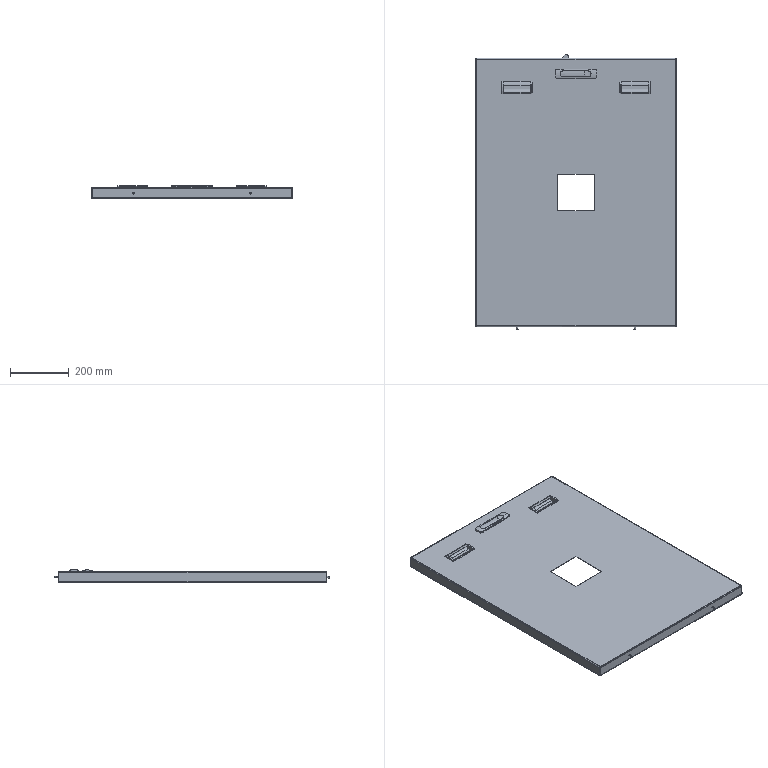Part | SolidWorks | 6 solids | 492 faces | box 685 x 936.5 x 44 mm | volume 1299683 mm3 | plane 226 | cylinder 188 | spline 46 | cone 26 | torus 6 | commonest cylinder face diameters 10 x27 2 x20 8.136 x15 6.6 x12 7 x11 3.242 x8